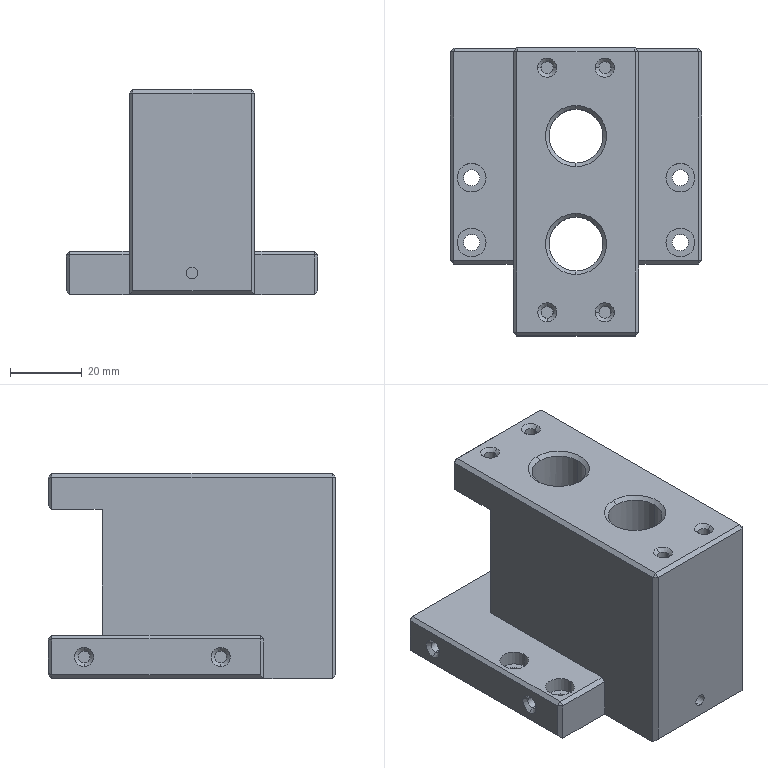Part | STEP file | Sensor fixing block-10P30 | 1 solid | 134 faces | box 70 x 80 x 57 mm | volume 133616 mm3 | plane 62 | cylinder 50 | cone 22 | commonest cylinder face diameters 3.3 x20 4.5 x8 8 x8 4 x6 15 x4 18 x2